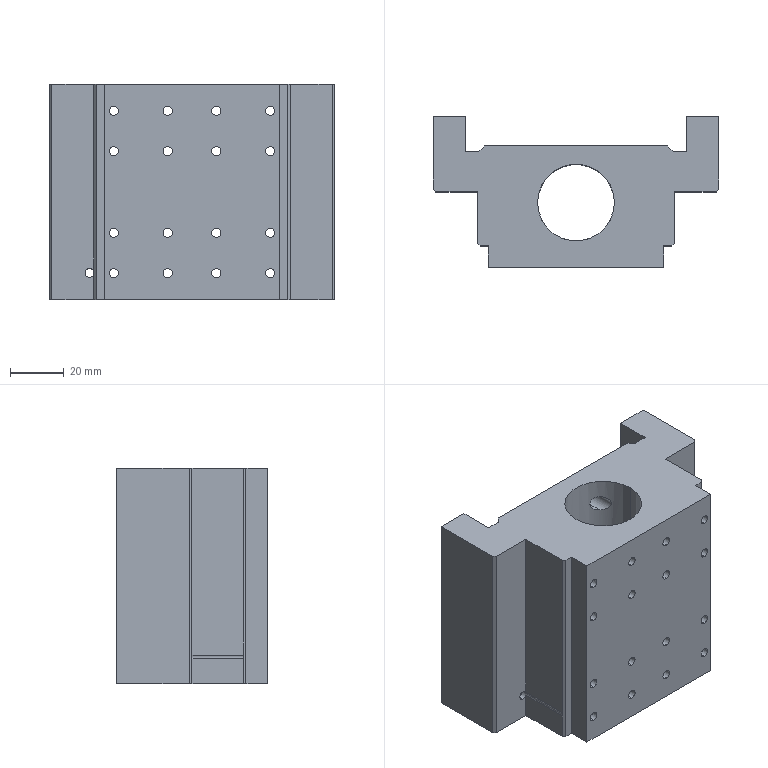Part | SolidWorks | features ICE 9, HoleWzd 7, Chamfer 4, CirPattern 2, Cut 2, Extrusion 1, LPattern 1 | 1 solid | 242 faces | box 106 x 56 x 80 mm | volume 252675 mm3 | cylinder 120 | plane 76 | cone 28 | spline 18 | commonest cylinder face diameters 6 x48 3.4 x32 4.2 x24 3.3 x8 2.5 x4 10 x2